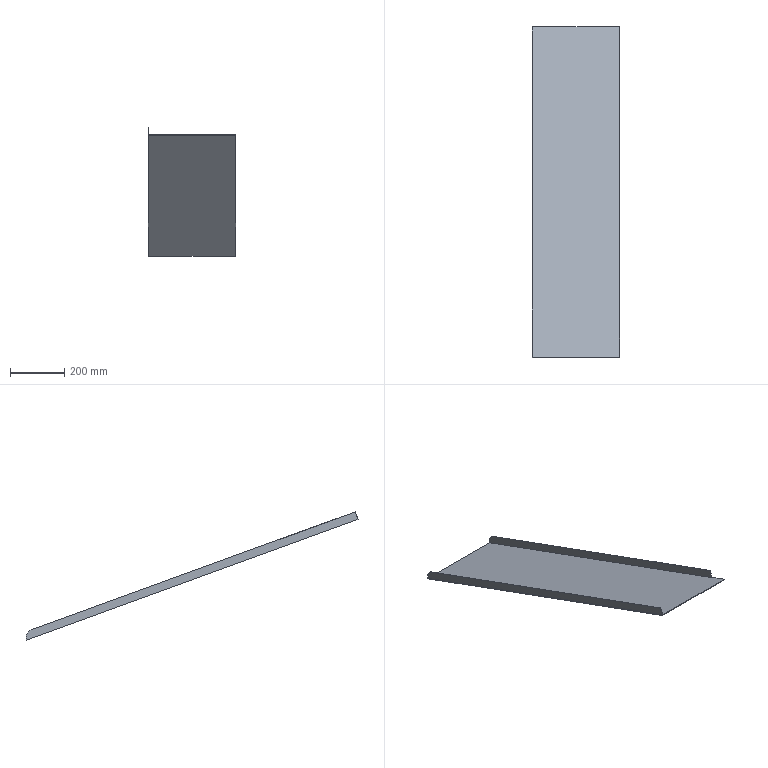Part | NX | features solid 2 | 1 solid | 13 faces | box 322.839 x 1223 x 472.565 mm | volume 979641 mm3 | plane 11 | cylinder 2 | commonest cylinder face diameters 60 x2
STEP:
#1=CARTESIAN_POINT('',(702.839,23.193,-196.203));
#2=VERTEX_POINT('',#1);
#3=CARTESIAN_POINT('',(702.839,-40.225,-173.121));
#4=VERTEX_POINT('',#3);
#5=CARTESIAN_POINT('',(702.839,-169.316,-126.135));
#6=DIRECTION('',(0.,-0.9397,0.342));
#7=VECTOR('',#6,1000.);
#8=LINE('',#5,#7);
#9=EDGE_CURVE('',#2,#4,#8,.T.);
#10=ORIENTED_EDGE('',*,*,#9,.F.);
#11=CARTESIAN_POINT('',(700.839,23.193,-196.203));
#12=VERTEX_POINT('',#11);
#13=CARTESIAN_POINT('',(45.,23.193,-196.203));
#14=DIRECTION('',(1.,0.,0.));
#15=VECTOR('',#14,1000.);
#16=LINE('',#13,#15);
#17=EDGE_CURVE('',#2,#12,#16,.F.);
#18=ORIENTED_EDGE('',*,*,#17,.T.);
#19=CARTESIAN_POINT('',(700.839,1180.,-617.246));
#20=VERTEX_POINT('',#19);
#21=CARTESIAN_POINT('',(700.839,-169.316,-126.135));
#22=DIRECTION('',(0.,-0.9397,0.342));
#23=VECTOR('',#22,1000.);
#24=LINE('',#21,#23);
#25=EDGE_CURVE('',#20,#12,#24,.T.);
#26=ORIENTED_EDGE('',*,*,#25,.F.);
#27=CARTESIAN_POINT('',(382.,1180.,-617.246));
#28=VERTEX_POINT('',#27);
#29=CARTESIAN_POINT('',(-625.,1180.,-617.246));
#30=DIRECTION('',(-1.,0.,0.));
#31=VECTOR('',#30,1000.);
#32=LINE('',#29,#31);
#33=EDGE_CURVE('',#28,#20,#32,.F.);
#34=ORIENTED_EDGE('',*,*,#33,.F.);
#35=CARTESIAN_POINT('',(382.,-40.225,-173.121));
#36=VERTEX_POINT('',#35);
#37=CARTESIAN_POINT('',(382.,-169.316,-126.135));
#38=DIRECTION('',(0.,-0.9397,0.342));
#39=VECTOR('',#38,1000.);
#40=LINE('',#37,#39);
#41=EDGE_CURVE('',#28,#36,#40,.T.);
#42=ORIENTED_EDGE('',*,*,#41,.T.);
#43=CARTESIAN_POINT('',(380.,-40.225,-173.121));
#44=DIRECTION('',(1.,0.,0.));
#45=VECTOR('',#44,1000.);
#46=LINE('',#43,#45);
#47=EDGE_CURVE('',#36,#4,#46,.T.);
#48=ORIENTED_EDGE('',*,*,#47,.T.);
#49=EDGE_LOOP('',(#10,#18,#26,#34,#42,#48));
#50=FACE_BOUND('',#49,.T.);
#51=CARTESIAN_POINT('',(45.,-169.316,-126.135));
#52=DIRECTION('',(0.,0.342,0.9397));
#53=DIRECTION('',(1.,0.,0.));
#54=AXIS2_PLACEMENT_3D('',#51,#52,#53);
#55=PLANE('',#54);
#56=ADVANCED_FACE('',(#50),#55,.T.);
#57=CARTESIAN_POINT('',(700.839,1180.,-619.375));
#58=VERTEX_POINT('',#57);
#59=CARTESIAN_POINT('',(700.839,1180.,-730.));
#60=DIRECTION('',(0.,0.,-1.));
#61=VECTOR('',#60,1000.);
#62=LINE('',#59,#61);
#63=EDGE_CURVE('',#58,#20,#62,.F.);
#64=ORIENTED_EDGE('',*,*,#63,.F.);
#65=CARTESIAN_POINT('',(382.,1180.,-619.375));
#66=VERTEX_POINT('',#65);
#67=CARTESIAN_POINT('',(-625.,1180.,-619.375));
#68=DIRECTION('',(-1.,0.,0.));
#69=VECTOR('',#68,1000.);
#70=LINE('',#67,#69);
#71=EDGE_CURVE('',#66,#58,#70,.F.);
#72=ORIENTED_EDGE('',*,*,#71,.F.);
#73=CARTESIAN_POINT('',(382.,1180.,-730.));
#74=DIRECTION('',(0.,0.,-1.));
#75=VECTOR('',#74,1000.);
#76=LINE('',#73,#75);
#77=EDGE_CURVE('',#66,#28,#76,.F.);
#78=ORIENTED_EDGE('',*,*,#77,.T.);
#79=ORIENTED_EDGE('',*,*,#33,.T.);
#80=EDGE_LOOP('',(#64,#72,#78,#79));
#81=FACE_BOUND('',#80,.T.);
#82=CARTESIAN_POINT('',(-625.,1180.,-730.));
#83=DIRECTION('',(0.,-1.,0.));
#84=DIRECTION('',(1.,0.,0.));
#85=AXIS2_PLACEMENT_3D('',#82,#83,#84);
#86=PLANE('',#85);
#87=ADVANCED_FACE('',(#81),#86,.F.);
#88=CARTESIAN_POINT('',(380.,1162.07,-580.923));
#89=VERTEX_POINT('',#88);
#90=CARTESIAN_POINT('',(380.,1180.,-619.375));
#91=VERTEX_POINT('',#90);
#92=CARTESIAN_POINT('',(380.,1151.809,-609.114));
#93=DIRECTION('',(-1.,0.,0.));
#94=DIRECTION('',(0.,-1.,0.));
#95=AXIS2_PLACEMENT_3D('',#92,#93,#94);
#96=CIRCLE('',#95,30.);
#97=EDGE_CURVE('',#89,#91,#96,.T.);
#98=ORIENTED_EDGE('',*,*,#97,.T.);
#99=CARTESIAN_POINT('',(380.,-40.909,-175.));
#100=VERTEX_POINT('',#99);
#101=CARTESIAN_POINT('',(380.,-170.,-128.015));
#102=DIRECTION('',(0.,-0.9397,0.342));
#103=VECTOR('',#102,1000.);
#104=LINE('',#101,#103);
#105=EDGE_CURVE('',#91,#100,#104,.T.);
#106=ORIENTED_EDGE('',*,*,#105,.T.);
#107=CARTESIAN_POINT('',(380.,-30.649,-146.809));
#108=VERTEX_POINT('',#107);
#109=CARTESIAN_POINT('',(380.,-40.225,-173.121));
#110=DIRECTION('',(0.,-0.342,-0.9397));
#111=VECTOR('',#110,1000.);
#112=LINE('',#109,#111);
#113=EDGE_CURVE('',#108,#100,#112,.T.);
#114=ORIENTED_EDGE('',*,*,#113,.F.);
#115=CARTESIAN_POINT('',(380.,1190.261,-591.184));
#116=DIRECTION('',(0.,-0.9397,0.342));
#117=VECTOR('',#116,1000.);
#118=LINE('',#115,#117);
#119=EDGE_CURVE('',#89,#108,#118,.T.);
#120=ORIENTED_EDGE('',*,*,#119,.F.);
#121=EDGE_LOOP('',(#98,#106,#114,#120));
#122=FACE_BOUND('',#121,.T.);
#123=CARTESIAN_POINT('',(380.,-169.316,-126.135));
#124=DIRECTION('',(1.,0.,0.));
#125=DIRECTION('',(0.,1.,0.));
#126=AXIS2_PLACEMENT_3D('',#123,#124,#125);
#127=PLANE('',#126);
#128=ADVANCED_FACE('',(#122),#127,.F.);
#129=CARTESIAN_POINT('',(702.839,-40.909,-175.));
#130=VERTEX_POINT('',#129);
#131=CARTESIAN_POINT('',(380.,-40.909,-175.));
#132=DIRECTION('',(1.,0.,0.));
#133=VECTOR('',#132,1000.);
#134=LINE('',#131,#133);
#135=EDGE_CURVE('',#100,#130,#134,.T.);
#136=ORIENTED_EDGE('',*,*,#135,.T.);
#137=CARTESIAN_POINT('',(702.839,-40.225,-173.121));
#138=DIRECTION('',(0.,-0.342,-0.9397));
#139=VECTOR('',#138,1000.);
#140=LINE('',#137,#139);
#141=EDGE_CURVE('',#4,#130,#140,.T.);
#142=ORIENTED_EDGE('',*,*,#141,.F.);
#143=ORIENTED_EDGE('',*,*,#47,.F.);
#144=CARTESIAN_POINT('',(382.,-30.649,-146.809));
#145=VERTEX_POINT('',#144);
#146=CARTESIAN_POINT('',(382.,-40.909,-175.));
#147=DIRECTION('',(0.,0.342,0.9397));
#148=VECTOR('',#147,1000.);
#149=LINE('',#146,#148);
#150=EDGE_CURVE('',#36,#145,#149,.T.);
#151=ORIENTED_EDGE('',*,*,#150,.T.);
#152=CARTESIAN_POINT('',(380.,-30.649,-146.809));
#153=DIRECTION('',(1.,0.,0.));
#154=VECTOR('',#153,1000.);
#155=LINE('',#152,#154);
#156=EDGE_CURVE('',#108,#145,#155,.T.);
#157=ORIENTED_EDGE('',*,*,#156,.F.);
#158=ORIENTED_EDGE('',*,*,#113,.T.);
#159=EDGE_LOOP('',(#136,#142,#143,#151,#157,#158));
#160=FACE_BOUND('',#159,.T.);
#161=CARTESIAN_POINT('',(380.,-40.225,-173.121));
#162=DIRECTION('',(0.,0.9397,-0.342));
#163=DIRECTION('',(0.,0.342,0.9397));
#164=AXIS2_PLACEMENT_3D('',#161,#162,#163);
#165=PLANE('',#164);
#166=ADVANCED_FACE('',(#160),#165,.F.);
#167=CARTESIAN_POINT('',(702.839,1180.,-619.375));
#168=VERTEX_POINT('',#167);
#169=CARTESIAN_POINT('',(702.839,-170.,-128.015));
#170=DIRECTION('',(0.,-0.9397,0.342));
#171=VECTOR('',#170,1000.);
#172=LINE('',#169,#171);
#173=EDGE_CURVE('',#168,#130,#172,.T.);
#174=ORIENTED_EDGE('',*,*,#173,.F.);
#175=CARTESIAN_POINT('',(702.839,1162.07,-580.923));
#176=VERTEX_POINT('',#175);
#177=CARTESIAN_POINT('',(702.839,1151.809,-609.114));
#178=DIRECTION('',(-1.,0.,0.));
#179=DIRECTION('',(0.,-1.,0.));
#180=AXIS2_PLACEMENT_3D('',#177,#178,#179);
#181=CIRCLE('',#180,30.);
#182=EDGE_CURVE('',#168,#176,#181,.F.);
#183=ORIENTED_EDGE('',*,*,#182,.T.);
#184=CARTESIAN_POINT('',(702.839,32.77,-169.892));
#185=VERTEX_POINT('',#184);
#186=CARTESIAN_POINT('',(702.839,1190.261,-591.184));
#187=DIRECTION('',(0.,-0.9397,0.342));
#188=VECTOR('',#187,1000.);
#189=LINE('',#186,#188);
#190=EDGE_CURVE('',#176,#185,#189,.T.);
#191=ORIENTED_EDGE('',*,*,#190,.T.);
#192=CARTESIAN_POINT('',(702.839,22.509,-198.083));
#193=DIRECTION('',(0.,0.342,0.9397));
#194=VECTOR('',#193,1000.);
#195=LINE('',#192,#194);
#196=EDGE_CURVE('',#2,#185,#195,.T.);
#197=ORIENTED_EDGE('',*,*,#196,.F.);
#198=ORIENTED_EDGE('',*,*,#9,.T.);
#199=ORIENTED_EDGE('',*,*,#141,.T.);
#200=EDGE_LOOP('',(#174,#183,#191,#197,#198,#199));
#201=FACE_BOUND('',#200,.T.);
#202=CARTESIAN_POINT('',(702.839,-169.316,-126.135));
#203=DIRECTION('',(1.,0.,0.));
#204=DIRECTION('',(0.,1.,0.));
#205=AXIS2_PLACEMENT_3D('',#202,#203,#204);
#206=PLANE('',#205);
#207=ADVANCED_FACE('',(#201),#206,.T.);
#208=CARTESIAN_POINT('',(702.839,1180.,-619.375));
#209=DIRECTION('',(1.,0.,0.));
#210=VECTOR('',#209,1000.);
#211=LINE('',#208,#210);
#212=EDGE_CURVE('',#168,#58,#211,.F.);
#213=ORIENTED_EDGE('',*,*,#212,.F.);
#214=ORIENTED_EDGE('',*,*,#173,.T.);
#215=ORIENTED_EDGE('',*,*,#135,.F.);
#216=ORIENTED_EDGE('',*,*,#105,.F.);
#217=CARTESIAN_POINT('',(-625.,1180.,-619.375));
#218=DIRECTION('',(-1.,0.,0.));
#219=VECTOR('',#218,1000.);
#220=LINE('',#217,#219);
#221=EDGE_CURVE('',#91,#66,#220,.F.);
#222=ORIENTED_EDGE('',*,*,#221,.T.);
#223=ORIENTED_EDGE('',*,*,#71,.T.);
#224=EDGE_LOOP('',(#213,#214,#215,#216,#222,#223));
#225=FACE_BOUND('',#224,.T.);
#226=CARTESIAN_POINT('',(45.,-170.,-128.015));
#227=DIRECTION('',(0.,0.342,0.9397));
#228=DIRECTION('',(1.,0.,0.));
#229=AXIS2_PLACEMENT_3D('',#226,#227,#228);
#230=PLANE('',#229);
#231=ADVANCED_FACE('',(#225),#230,.F.);
#232=CARTESIAN_POINT('',(382.,1162.07,-580.923));
#233=VERTEX_POINT('',#232);
#234=CARTESIAN_POINT('',(382.,1190.261,-591.184));
#235=DIRECTION('',(0.,-0.9397,0.342));
#236=VECTOR('',#235,1000.);
#237=LINE('',#234,#236);
#238=EDGE_CURVE('',#233,#145,#237,.T.);
#239=ORIENTED_EDGE('',*,*,#238,.F.);
#240=CARTESIAN_POINT('',(380.,1162.07,-580.923));
#241=DIRECTION('',(-1.,0.,0.));
#242=VECTOR('',#241,1000.);
#243=LINE('',#240,#242);
#244=EDGE_CURVE('',#233,#89,#243,.T.);
#245=ORIENTED_EDGE('',*,*,#244,.T.);
#246=ORIENTED_EDGE('',*,*,#119,.T.);
#247=ORIENTED_EDGE('',*,*,#156,.T.);
#248=EDGE_LOOP('',(#239,#245,#246,#247));
#249=FACE_BOUND('',#248,.T.);
#250=CARTESIAN_POINT('',(380.,1190.261,-591.184));
#251=DIRECTION('',(0.,-0.342,-0.9397));
#252=DIRECTION('',(0.,-0.9397,0.342));
#253=AXIS2_PLACEMENT_3D('',#250,#251,#252);
#254=PLANE('',#253);
#255=ADVANCED_FACE('',(#249),#254,.F.);
#256=ORIENTED_EDGE('',*,*,#77,.F.);
#257=CARTESIAN_POINT('',(382.,1151.809,-609.114));
#258=DIRECTION('',(-1.,0.,0.));
#259=DIRECTION('',(0.,-1.,0.));
#260=AXIS2_PLACEMENT_3D('',#257,#258,#259);
#261=CIRCLE('',#260,30.);
#262=EDGE_CURVE('',#66,#233,#261,.F.);
#263=ORIENTED_EDGE('',*,*,#262,.T.);
#264=ORIENTED_EDGE('',*,*,#238,.T.);
#265=ORIENTED_EDGE('',*,*,#150,.F.);
#266=ORIENTED_EDGE('',*,*,#41,.F.);
#267=EDGE_LOOP('',(#256,#263,#264,#265,#266));
#268=FACE_BOUND('',#267,.T.);
#269=CARTESIAN_POINT('',(382.,1180.,-619.375));
#270=DIRECTION('',(-1.,0.,0.));
#271=DIRECTION('',(0.,-1.,0.));
#272=AXIS2_PLACEMENT_3D('',#269,#270,#271);
#273=PLANE('',#272);
#274=ADVANCED_FACE('',(#268),#273,.F.);
#275=ORIENTED_EDGE('',*,*,#97,.F.);
#276=ORIENTED_EDGE('',*,*,#244,.F.);
#277=ORIENTED_EDGE('',*,*,#262,.F.);
#278=ORIENTED_EDGE('',*,*,#221,.F.);
#279=EDGE_LOOP('',(#275,#276,#277,#278));
#280=FACE_BOUND('',#279,.T.);
#281=CARTESIAN_POINT('',(380.,1151.809,-609.114));
#282=DIRECTION('',(1.,0.,0.));
#283=DIRECTION('',(0.,1.,0.));
#284=AXIS2_PLACEMENT_3D('',#281,#282,#283);
#285=CYLINDRICAL_SURFACE('',#284,30.);
#286=ADVANCED_FACE('',(#280),#285,.T.);
#287=ORIENTED_EDGE('',*,*,#190,.F.);
#288=CARTESIAN_POINT('',(700.839,1162.07,-580.923));
#289=VERTEX_POINT('',#288);
#290=CARTESIAN_POINT('',(702.839,1162.07,-580.923));
#291=DIRECTION('',(-1.,0.,0.));
#292=VECTOR('',#291,1000.);
#293=LINE('',#290,#292);
#294=EDGE_CURVE('',#176,#289,#293,.T.);
#295=ORIENTED_EDGE('',*,*,#294,.T.);
#296=CARTESIAN_POINT('',(700.839,32.77,-169.892));
#297=VERTEX_POINT('',#296);
#298=CARTESIAN_POINT('',(700.839,1190.261,-591.184));
#299=DIRECTION('',(0.,-0.9397,0.342));
#300=VECTOR('',#299,1000.);
#301=LINE('',#298,#300);
#302=EDGE_CURVE('',#289,#297,#301,.T.);
#303=ORIENTED_EDGE('',*,*,#302,.T.);
#304=CARTESIAN_POINT('',(702.839,32.77,-169.892));
#305=DIRECTION('',(1.,0.,0.));
#306=VECTOR('',#305,1000.);
#307=LINE('',#304,#306);
#308=EDGE_CURVE('',#185,#297,#307,.F.);
#309=ORIENTED_EDGE('',*,*,#308,.F.);
#310=EDGE_LOOP('',(#287,#295,#303,#309));
#311=FACE_BOUND('',#310,.T.);
#312=CARTESIAN_POINT('',(702.839,1190.261,-591.184));
#313=DIRECTION('',(0.,-0.342,-0.9397));
#314=DIRECTION('',(0.,-0.9397,0.342));
#315=AXIS2_PLACEMENT_3D('',#312,#313,#314);
#316=PLANE('',#315);
#317=ADVANCED_FACE('',(#311),#316,.F.);
#318=ORIENTED_EDGE('',*,*,#17,.F.);
#319=ORIENTED_EDGE('',*,*,#196,.T.);
#320=ORIENTED_EDGE('',*,*,#308,.T.);
#321=CARTESIAN_POINT('',(700.839,22.509,-198.083));
#322=DIRECTION('',(0.,0.342,0.9397));
#323=VECTOR('',#322,1000.);
#324=LINE('',#321,#323);
#325=EDGE_CURVE('',#12,#297,#324,.T.);
#326=ORIENTED_EDGE('',*,*,#325,.F.);
#327=EDGE_LOOP('',(#318,#319,#320,#326));
#328=FACE_BOUND('',#327,.T.);
#329=CARTESIAN_POINT('',(702.839,22.509,-198.083));
#330=DIRECTION('',(0.,-0.9397,0.342));
#331=DIRECTION('',(0.,0.342,0.9397));
#332=AXIS2_PLACEMENT_3D('',#329,#330,#331);
#333=PLANE('',#332);
#334=ADVANCED_FACE('',(#328),#333,.T.);
#335=CARTESIAN_POINT('',(700.839,1151.809,-609.114));
#336=DIRECTION('',(-1.,0.,0.));
#337=DIRECTION('',(0.,-1.,0.));
#338=AXIS2_PLACEMENT_3D('',#335,#336,#337);
#339=CIRCLE('',#338,30.);
#340=EDGE_CURVE('',#289,#58,#339,.T.);
#341=ORIENTED_EDGE('',*,*,#340,.T.);
#342=ORIENTED_EDGE('',*,*,#63,.T.);
#343=ORIENTED_EDGE('',*,*,#25,.T.);
#344=ORIENTED_EDGE('',*,*,#325,.T.);
#345=ORIENTED_EDGE('',*,*,#302,.F.);
#346=EDGE_LOOP('',(#341,#342,#343,#344,#345));
#347=FACE_BOUND('',#346,.T.);
#348=CARTESIAN_POINT('',(700.839,1180.,-619.375));
#349=DIRECTION('',(-1.,0.,0.));
#350=DIRECTION('',(0.,-1.,0.));
#351=AXIS2_PLACEMENT_3D('',#348,#349,#350);
#352=PLANE('',#351);
#353=ADVANCED_FACE('',(#347),#352,.T.);
#354=ORIENTED_EDGE('',*,*,#182,.F.);
#355=ORIENTED_EDGE('',*,*,#212,.T.);
#356=ORIENTED_EDGE('',*,*,#340,.F.);
#357=ORIENTED_EDGE('',*,*,#294,.F.);
#358=EDGE_LOOP('',(#354,#355,#356,#357));
#359=FACE_BOUND('',#358,.T.);
#360=CARTESIAN_POINT('',(702.839,1151.809,-609.114));
#361=DIRECTION('',(-1.,0.,0.));
#362=DIRECTION('',(0.,-1.,0.));
#363=AXIS2_PLACEMENT_3D('',#360,#361,#362);
#364=CYLINDRICAL_SURFACE('',#363,30.);
#365=ADVANCED_FACE('',(#359),#364,.T.);
#366=CLOSED_SHELL('',(#56,#87,#128,#166,#207,#231,#255,#274,#286,#317,#334,#353,#365));
#367=MANIFOLD_SOLID_BREP('',#366);
#368=(LENGTH_UNIT()NAMED_UNIT(*)SI_UNIT(.MILLI.,.METRE.));
#369=UNCERTAINTY_MEASURE_WITH_UNIT(LENGTH_MEASURE(0.0508),#368,'','');
#370=(NAMED_UNIT(*)PLANE_ANGLE_UNIT()SI_UNIT($,.RADIAN.));
#371=(NAMED_UNIT(*)SI_UNIT($,.STERADIAN.)SOLID_ANGLE_UNIT());
#372=(GEOMETRIC_REPRESENTATION_CONTEXT(3)GLOBAL_UNCERTAINTY_ASSIGNED_CONTEXT((#369))GLOBAL_UNIT_ASSIGNED_CONTEXT((#368,#370,#371))REPRESENTATION_CONTEXT('',''));
#373=ADVANCED_BREP_SHAPE_REPRESENTATION('',(#367),#372);